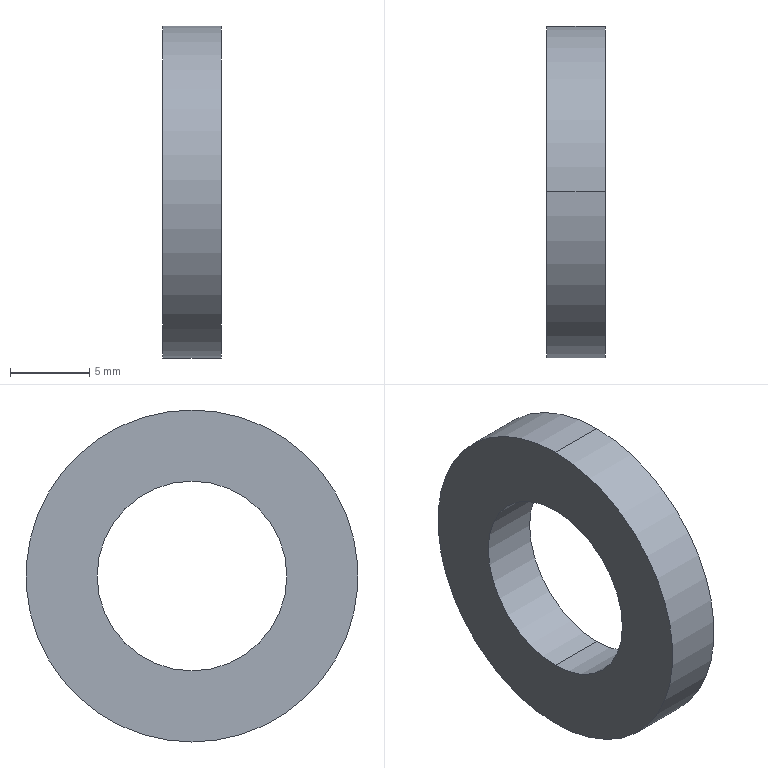Part | STEP file | LHBBW12collar3_Default | 1 solid | 6 faces | box 3.7 x 21 x 21 mm | volume 863.074 mm3 | cylinder 4 | plane 2 | commonest cylinder face diameters 12 x2 21 x2
STEP:
#1=CARTESIAN_POINT('',(0.,0.,0.));
#2=DIRECTION('',(0.,0.,1.));
#3=DIRECTION('',(1.,0.,0.));
#4=AXIS2_PLACEMENT_3D('',#1,#2,#3);
#5=CARTESIAN_POINT('',(1.85,0.,6.));
#6=VERTEX_POINT('',#5);
#7=CARTESIAN_POINT('',(-1.85,0.,6.));
#8=VERTEX_POINT('',#7);
#9=CARTESIAN_POINT('',(1.85,0.,6.));
#10=DIRECTION('',(-1.,0.,0.));
#11=VECTOR('',#10,1.);
#12=LINE('',#9,#11);
#13=CARTESIAN_POINT('',(1.85,0.,0.));
#14=DIRECTION('',(-1.,0.,0.));
#15=DIRECTION('',(0.,0.,1.));
#16=AXIS2_PLACEMENT_3D('',#13,#14,#15);
#17=CYLINDRICAL_SURFACE('',#16,6.);
#18=CARTESIAN_POINT('',(6.283,0.));
#19=DIRECTION('',(0.,1.));
#20=VECTOR('',#19,1.);
#21=LINE('',#18,#20);
#22=(GEOMETRIC_REPRESENTATION_CONTEXT(2)PARAMETRIC_REPRESENTATION_CONTEXT()REPRESENTATION_CONTEXT('',''));
#23=DEFINITIONAL_REPRESENTATION('',(#21),#22);
#24=PCURVE('',#17,#23);
#25=CARTESIAN_POINT('',(1.85,0.,0.));
#26=DIRECTION('',(-1.,0.,0.));
#27=DIRECTION('',(0.,0.,1.));
#28=AXIS2_PLACEMENT_3D('',#25,#26,#27);
#29=CYLINDRICAL_SURFACE('',#28,6.);
#30=CARTESIAN_POINT('',(0.,0.));
#31=DIRECTION('',(0.,1.));
#32=VECTOR('',#31,1.);
#33=LINE('',#30,#32);
#34=(GEOMETRIC_REPRESENTATION_CONTEXT(2)PARAMETRIC_REPRESENTATION_CONTEXT()REPRESENTATION_CONTEXT('',''));
#35=DEFINITIONAL_REPRESENTATION('',(#33),#34);
#36=PCURVE('',#29,#35);
#37=SURFACE_CURVE('',#12,(#24,#36),.PCURVE_S1.);
#38=EDGE_CURVE('',#6,#8,#37,.T.);
#39=ORIENTED_EDGE('',*,*,#38,.T.);
#40=CARTESIAN_POINT('',(-1.85,0.,-6.));
#41=VERTEX_POINT('',#40);
#42=CARTESIAN_POINT('',(-1.85,0.,0.));
#43=DIRECTION('',(-1.,0.,0.));
#44=DIRECTION('',(0.,0.,1.));
#45=AXIS2_PLACEMENT_3D('',#42,#43,#44);
#46=CIRCLE('',#45,6.);
#47=CARTESIAN_POINT('',(0.,3.7));
#48=DIRECTION('',(1.,0.));
#49=VECTOR('',#48,1.);
#50=LINE('',#47,#49);
#51=(GEOMETRIC_REPRESENTATION_CONTEXT(2)PARAMETRIC_REPRESENTATION_CONTEXT()REPRESENTATION_CONTEXT('',''));
#52=DEFINITIONAL_REPRESENTATION('',(#50),#51);
#53=PCURVE('',#17,#52);
#54=CARTESIAN_POINT('',(-1.85,10.5,0.));
#55=DIRECTION('',(1.,0.,0.));
#56=DIRECTION('',(0.,0.,-1.));
#57=AXIS2_PLACEMENT_3D('',#54,#55,#56);
#58=PLANE('',#57);
#59=CARTESIAN_POINT('',(-6.,-10.5));
#60=CARTESIAN_POINT('',(-6.,-0.1077));
#61=CARTESIAN_POINT('',(3.,-5.304));
#62=CARTESIAN_POINT('',(12.,-10.5));
#63=CARTESIAN_POINT('',(3.,-15.696));
#64=CARTESIAN_POINT('',(-6.,-20.892));
#65=CARTESIAN_POINT('',(-6.,-10.5));
#66=(BOUNDED_CURVE()B_SPLINE_CURVE(2,(#59,#60,#61,#62,#63,#64,#65),.UNSPECIFIED.,.T.,.F.)B_SPLINE_CURVE_WITH_KNOTS((1,2,2,2,2,1),(-2.094,0.,2.094,4.189,6.283,8.378),.UNSPECIFIED.)CURVE()GEOMETRIC_REPRESENTATION_ITEM()RATIONAL_B_SPLINE_CURVE((1.,0.5,1.,0.5,1.,0.5,1.))REPRESENTATION_ITEM(''));
#67=(GEOMETRIC_REPRESENTATION_CONTEXT(2)PARAMETRIC_REPRESENTATION_CONTEXT()REPRESENTATION_CONTEXT('',''));
#68=DEFINITIONAL_REPRESENTATION('',(#66),#67);
#69=PCURVE('',#58,#68);
#70=SURFACE_CURVE('',#46,(#53,#69),.PCURVE_S1.);
#71=EDGE_CURVE('',#41,#8,#70,.T.);
#72=ORIENTED_EDGE('',*,*,#71,.F.);
#73=CARTESIAN_POINT('',(1.85,0.,-6.));
#74=VERTEX_POINT('',#73);
#75=CARTESIAN_POINT('',(1.85,0.,-6.));
#76=DIRECTION('',(-1.,0.,0.));
#77=VECTOR('',#76,1.);
#78=LINE('',#75,#77);
#79=CARTESIAN_POINT('',(3.142,0.));
#80=DIRECTION('',(0.,1.));
#81=VECTOR('',#80,1.);
#82=LINE('',#79,#81);
#83=(GEOMETRIC_REPRESENTATION_CONTEXT(2)PARAMETRIC_REPRESENTATION_CONTEXT()REPRESENTATION_CONTEXT('',''));
#84=DEFINITIONAL_REPRESENTATION('',(#82),#83);
#85=PCURVE('',#17,#84);
#86=CARTESIAN_POINT('',(3.142,0.));
#87=DIRECTION('',(0.,1.));
#88=VECTOR('',#87,1.);
#89=LINE('',#86,#88);
#90=(GEOMETRIC_REPRESENTATION_CONTEXT(2)PARAMETRIC_REPRESENTATION_CONTEXT()REPRESENTATION_CONTEXT('',''));
#91=DEFINITIONAL_REPRESENTATION('',(#89),#90);
#92=PCURVE('',#29,#91);
#93=SURFACE_CURVE('',#78,(#85,#92),.PCURVE_S1.);
#94=EDGE_CURVE('',#74,#41,#93,.T.);
#95=ORIENTED_EDGE('',*,*,#94,.F.);
#96=CARTESIAN_POINT('',(1.85,0.,0.));
#97=DIRECTION('',(-1.,0.,0.));
#98=DIRECTION('',(0.,0.,1.));
#99=AXIS2_PLACEMENT_3D('',#96,#97,#98);
#100=CIRCLE('',#99,6.);
#101=CARTESIAN_POINT('',(0.,0.));
#102=DIRECTION('',(1.,0.));
#103=VECTOR('',#102,1.);
#104=LINE('',#101,#103);
#105=(GEOMETRIC_REPRESENTATION_CONTEXT(2)PARAMETRIC_REPRESENTATION_CONTEXT()REPRESENTATION_CONTEXT('',''));
#106=DEFINITIONAL_REPRESENTATION('',(#104),#105);
#107=PCURVE('',#17,#106);
#108=CARTESIAN_POINT('',(1.85,6.,0.));
#109=DIRECTION('',(-1.,0.,0.));
#110=DIRECTION('',(0.,0.,1.));
#111=AXIS2_PLACEMENT_3D('',#108,#109,#110);
#112=PLANE('',#111);
#113=CARTESIAN_POINT('',(0.,-6.));
#114=DIRECTION('',(1.,0.));
#115=AXIS2_PLACEMENT_2D('',#113,#114);
#116=CIRCLE('',#115,6.);
#117=(GEOMETRIC_REPRESENTATION_CONTEXT(2)PARAMETRIC_REPRESENTATION_CONTEXT()REPRESENTATION_CONTEXT('',''));
#118=DEFINITIONAL_REPRESENTATION('',(#116),#117);
#119=PCURVE('',#112,#118);
#120=SURFACE_CURVE('',#100,(#107,#119),.PCURVE_S1.);
#121=EDGE_CURVE('',#74,#6,#120,.T.);
#122=ORIENTED_EDGE('',*,*,#121,.T.);
#123=EDGE_LOOP('',(#39,#72,#95,#122));
#124=FACE_BOUND('',#123,.F.);
#125=ADVANCED_FACE('',(#124),#17,.F.);
#126=CARTESIAN_POINT('',(1.85,0.,10.5));
#127=VERTEX_POINT('',#126);
#128=CARTESIAN_POINT('',(1.85,0.,-10.5));
#129=VERTEX_POINT('',#128);
#130=CARTESIAN_POINT('',(1.85,0.,0.));
#131=DIRECTION('',(-1.,0.,0.));
#132=DIRECTION('',(0.,0.,1.));
#133=AXIS2_PLACEMENT_3D('',#130,#131,#132);
#134=CIRCLE('',#133,10.5);
#135=CARTESIAN_POINT('',(1.85,0.,0.));
#136=DIRECTION('',(-1.,0.,0.));
#137=DIRECTION('',(0.,0.,1.));
#138=AXIS2_PLACEMENT_3D('',#135,#136,#137);
#139=CYLINDRICAL_SURFACE('',#138,10.5);
#140=CARTESIAN_POINT('',(0.,0.));
#141=DIRECTION('',(1.,0.));
#142=VECTOR('',#141,1.);
#143=LINE('',#140,#142);
#144=(GEOMETRIC_REPRESENTATION_CONTEXT(2)PARAMETRIC_REPRESENTATION_CONTEXT()REPRESENTATION_CONTEXT('',''));
#145=DEFINITIONAL_REPRESENTATION('',(#143),#144);
#146=PCURVE('',#139,#145);
#147=CARTESIAN_POINT('',(0.,-6.));
#148=DIRECTION('',(1.,0.));
#149=AXIS2_PLACEMENT_2D('',#147,#148);
#150=CIRCLE('',#149,10.5);
#151=(GEOMETRIC_REPRESENTATION_CONTEXT(2)PARAMETRIC_REPRESENTATION_CONTEXT()REPRESENTATION_CONTEXT('',''));
#152=DEFINITIONAL_REPRESENTATION('',(#150),#151);
#153=PCURVE('',#112,#152);
#154=SURFACE_CURVE('',#134,(#146,#153),.PCURVE_S1.);
#155=EDGE_CURVE('',#127,#129,#154,.T.);
#156=ORIENTED_EDGE('',*,*,#155,.T.);
#157=CARTESIAN_POINT('',(-1.85,0.,-10.5));
#158=VERTEX_POINT('',#157);
#159=CARTESIAN_POINT('',(1.85,0.,-10.5));
#160=DIRECTION('',(-1.,0.,0.));
#161=VECTOR('',#160,1.);
#162=LINE('',#159,#161);
#163=CARTESIAN_POINT('',(3.142,0.));
#164=DIRECTION('',(0.,1.));
#165=VECTOR('',#164,1.);
#166=LINE('',#163,#165);
#167=(GEOMETRIC_REPRESENTATION_CONTEXT(2)PARAMETRIC_REPRESENTATION_CONTEXT()REPRESENTATION_CONTEXT('',''));
#168=DEFINITIONAL_REPRESENTATION('',(#166),#167);
#169=PCURVE('',#139,#168);
#170=CARTESIAN_POINT('',(1.85,0.,0.));
#171=DIRECTION('',(-1.,0.,0.));
#172=DIRECTION('',(0.,0.,1.));
#173=AXIS2_PLACEMENT_3D('',#170,#171,#172);
#174=CYLINDRICAL_SURFACE('',#173,10.5);
#175=CARTESIAN_POINT('',(3.142,0.));
#176=DIRECTION('',(0.,1.));
#177=VECTOR('',#176,1.);
#178=LINE('',#175,#177);
#179=(GEOMETRIC_REPRESENTATION_CONTEXT(2)PARAMETRIC_REPRESENTATION_CONTEXT()REPRESENTATION_CONTEXT('',''));
#180=DEFINITIONAL_REPRESENTATION('',(#178),#179);
#181=PCURVE('',#174,#180);
#182=SURFACE_CURVE('',#162,(#169,#181),.PCURVE_S1.);
#183=EDGE_CURVE('',#129,#158,#182,.T.);
#184=ORIENTED_EDGE('',*,*,#183,.T.);
#185=CARTESIAN_POINT('',(-1.85,0.,10.5));
#186=VERTEX_POINT('',#185);
#187=CARTESIAN_POINT('',(-1.85,0.,0.));
#188=DIRECTION('',(-1.,0.,0.));
#189=DIRECTION('',(0.,0.,1.));
#190=AXIS2_PLACEMENT_3D('',#187,#188,#189);
#191=CIRCLE('',#190,10.5);
#192=CARTESIAN_POINT('',(0.,3.7));
#193=DIRECTION('',(1.,0.));
#194=VECTOR('',#193,1.);
#195=LINE('',#192,#194);
#196=(GEOMETRIC_REPRESENTATION_CONTEXT(2)PARAMETRIC_REPRESENTATION_CONTEXT()REPRESENTATION_CONTEXT('',''));
#197=DEFINITIONAL_REPRESENTATION('',(#195),#196);
#198=PCURVE('',#139,#197);
#199=CARTESIAN_POINT('',(-10.5,-10.5));
#200=CARTESIAN_POINT('',(-10.5,7.687));
#201=CARTESIAN_POINT('',(5.25,-1.407));
#202=CARTESIAN_POINT('',(21.,-10.5));
#203=CARTESIAN_POINT('',(5.25,-19.593));
#204=CARTESIAN_POINT('',(-10.5,-28.687));
#205=CARTESIAN_POINT('',(-10.5,-10.5));
#206=(BOUNDED_CURVE()B_SPLINE_CURVE(2,(#199,#200,#201,#202,#203,#204,#205),.UNSPECIFIED.,.T.,.F.)B_SPLINE_CURVE_WITH_KNOTS((1,2,2,2,2,1),(-2.094,0.,2.094,4.189,6.283,8.378),.UNSPECIFIED.)CURVE()GEOMETRIC_REPRESENTATION_ITEM()RATIONAL_B_SPLINE_CURVE((1.,0.5,1.,0.5,1.,0.5,1.))REPRESENTATION_ITEM(''));
#207=(GEOMETRIC_REPRESENTATION_CONTEXT(2)PARAMETRIC_REPRESENTATION_CONTEXT()REPRESENTATION_CONTEXT('',''));
#208=DEFINITIONAL_REPRESENTATION('',(#206),#207);
#209=PCURVE('',#58,#208);
#210=SURFACE_CURVE('',#191,(#198,#209),.PCURVE_S1.);
#211=EDGE_CURVE('',#186,#158,#210,.T.);
#212=ORIENTED_EDGE('',*,*,#211,.F.);
#213=CARTESIAN_POINT('',(1.85,0.,10.5));
#214=DIRECTION('',(-1.,0.,0.));
#215=VECTOR('',#214,1.);
#216=LINE('',#213,#215);
#217=CARTESIAN_POINT('',(0.,0.));
#218=DIRECTION('',(0.,1.));
#219=VECTOR('',#218,1.);
#220=LINE('',#217,#219);
#221=(GEOMETRIC_REPRESENTATION_CONTEXT(2)PARAMETRIC_REPRESENTATION_CONTEXT()REPRESENTATION_CONTEXT('',''));
#222=DEFINITIONAL_REPRESENTATION('',(#220),#221);
#223=PCURVE('',#139,#222);
#224=CARTESIAN_POINT('',(6.283,0.));
#225=DIRECTION('',(0.,1.));
#226=VECTOR('',#225,1.);
#227=LINE('',#224,#226);
#228=(GEOMETRIC_REPRESENTATION_CONTEXT(2)PARAMETRIC_REPRESENTATION_CONTEXT()REPRESENTATION_CONTEXT('',''));
#229=DEFINITIONAL_REPRESENTATION('',(#227),#228);
#230=PCURVE('',#174,#229);
#231=SURFACE_CURVE('',#216,(#223,#230),.PCURVE_S1.);
#232=EDGE_CURVE('',#127,#186,#231,.T.);
#233=ORIENTED_EDGE('',*,*,#232,.F.);
#234=EDGE_LOOP('',(#156,#184,#212,#233));
#235=FACE_BOUND('',#234,.T.);
#236=ADVANCED_FACE('',(#235),#139,.T.);
#237=ORIENTED_EDGE('',*,*,#183,.F.);
#238=CARTESIAN_POINT('',(1.85,0.,0.));
#239=DIRECTION('',(-1.,0.,0.));
#240=DIRECTION('',(0.,0.,1.));
#241=AXIS2_PLACEMENT_3D('',#238,#239,#240);
#242=CIRCLE('',#241,10.5);
#243=CARTESIAN_POINT('',(0.,0.));
#244=DIRECTION('',(1.,0.));
#245=VECTOR('',#244,1.);
#246=LINE('',#243,#245);
#247=(GEOMETRIC_REPRESENTATION_CONTEXT(2)PARAMETRIC_REPRESENTATION_CONTEXT()REPRESENTATION_CONTEXT('',''));
#248=DEFINITIONAL_REPRESENTATION('',(#246),#247);
#249=PCURVE('',#174,#248);
#250=CARTESIAN_POINT('',(0.,-6.));
#251=DIRECTION('',(1.,0.));
#252=AXIS2_PLACEMENT_2D('',#250,#251);
#253=CIRCLE('',#252,10.5);
#254=(GEOMETRIC_REPRESENTATION_CONTEXT(2)PARAMETRIC_REPRESENTATION_CONTEXT()REPRESENTATION_CONTEXT('',''));
#255=DEFINITIONAL_REPRESENTATION('',(#253),#254);
#256=PCURVE('',#112,#255);
#257=SURFACE_CURVE('',#242,(#249,#256),.PCURVE_S1.);
#258=EDGE_CURVE('',#129,#127,#257,.T.);
#259=ORIENTED_EDGE('',*,*,#258,.T.);
#260=ORIENTED_EDGE('',*,*,#232,.T.);
#261=CARTESIAN_POINT('',(-1.85,0.,0.));
#262=DIRECTION('',(-1.,0.,0.));
#263=DIRECTION('',(0.,0.,1.));
#264=AXIS2_PLACEMENT_3D('',#261,#262,#263);
#265=CIRCLE('',#264,10.5);
#266=CARTESIAN_POINT('',(0.,3.7));
#267=DIRECTION('',(1.,0.));
#268=VECTOR('',#267,1.);
#269=LINE('',#266,#268);
#270=(GEOMETRIC_REPRESENTATION_CONTEXT(2)PARAMETRIC_REPRESENTATION_CONTEXT()REPRESENTATION_CONTEXT('',''));
#271=DEFINITIONAL_REPRESENTATION('',(#269),#270);
#272=PCURVE('',#174,#271);
#273=CARTESIAN_POINT('',(-10.5,-10.5));
#274=CARTESIAN_POINT('',(-10.5,7.687));
#275=CARTESIAN_POINT('',(5.25,-1.407));
#276=CARTESIAN_POINT('',(21.,-10.5));
#277=CARTESIAN_POINT('',(5.25,-19.593));
#278=CARTESIAN_POINT('',(-10.5,-28.687));
#279=CARTESIAN_POINT('',(-10.5,-10.5));
#280=(BOUNDED_CURVE()B_SPLINE_CURVE(2,(#273,#274,#275,#276,#277,#278,#279),.UNSPECIFIED.,.T.,.F.)B_SPLINE_CURVE_WITH_KNOTS((1,2,2,2,2,1),(-2.094,0.,2.094,4.189,6.283,8.378),.UNSPECIFIED.)CURVE()GEOMETRIC_REPRESENTATION_ITEM()RATIONAL_B_SPLINE_CURVE((1.,0.5,1.,0.5,1.,0.5,1.))REPRESENTATION_ITEM(''));
#281=(GEOMETRIC_REPRESENTATION_CONTEXT(2)PARAMETRIC_REPRESENTATION_CONTEXT()REPRESENTATION_CONTEXT('',''));
#282=DEFINITIONAL_REPRESENTATION('',(#280),#281);
#283=PCURVE('',#58,#282);
#284=SURFACE_CURVE('',#265,(#272,#283),.PCURVE_S1.);
#285=EDGE_CURVE('',#158,#186,#284,.T.);
#286=ORIENTED_EDGE('',*,*,#285,.F.);
#287=EDGE_LOOP('',(#237,#259,#260,#286));
#288=FACE_BOUND('',#287,.T.);
#289=ADVANCED_FACE('',(#288),#174,.T.);
#290=CARTESIAN_POINT('',(-1.85,0.,0.));
#291=DIRECTION('',(-1.,0.,0.));
#292=DIRECTION('',(0.,0.,1.));
#293=AXIS2_PLACEMENT_3D('',#290,#291,#292);
#294=CIRCLE('',#293,6.);
#295=CARTESIAN_POINT('',(-6.,-10.5));
#296=CARTESIAN_POINT('',(-6.,-0.1077));
#297=CARTESIAN_POINT('',(3.,-5.304));
#298=CARTESIAN_POINT('',(12.,-10.5));
#299=CARTESIAN_POINT('',(3.,-15.696));
#300=CARTESIAN_POINT('',(-6.,-20.892));
#301=CARTESIAN_POINT('',(-6.,-10.5));
#302=(BOUNDED_CURVE()B_SPLINE_CURVE(2,(#295,#296,#297,#298,#299,#300,#301),.UNSPECIFIED.,.T.,.F.)B_SPLINE_CURVE_WITH_KNOTS((1,2,2,2,2,1),(-2.094,0.,2.094,4.189,6.283,8.378),.UNSPECIFIED.)CURVE()GEOMETRIC_REPRESENTATION_ITEM()RATIONAL_B_SPLINE_CURVE((1.,0.5,1.,0.5,1.,0.5,1.))REPRESENTATION_ITEM(''));
#303=(GEOMETRIC_REPRESENTATION_CONTEXT(2)PARAMETRIC_REPRESENTATION_CONTEXT()REPRESENTATION_CONTEXT('',''));
#304=DEFINITIONAL_REPRESENTATION('',(#302),#303);
#305=PCURVE('',#58,#304);
#306=CARTESIAN_POINT('',(0.,3.7));
#307=DIRECTION('',(1.,0.));
#308=VECTOR('',#307,1.);
#309=LINE('',#306,#308);
#310=(GEOMETRIC_REPRESENTATION_CONTEXT(2)PARAMETRIC_REPRESENTATION_CONTEXT()REPRESENTATION_CONTEXT('',''));
#311=DEFINITIONAL_REPRESENTATION('',(#309),#310);
#312=PCURVE('',#29,#311);
#313=SURFACE_CURVE('',#294,(#305,#312),.PCURVE_S1.);
#314=EDGE_CURVE('',#8,#41,#313,.T.);
#315=ORIENTED_EDGE('',*,*,#314,.F.);
#316=ORIENTED_EDGE('',*,*,#71,.F.);
#317=EDGE_LOOP('',(#315,#316));
#318=FACE_BOUND('',#317,.T.);
#319=ORIENTED_EDGE('',*,*,#211,.T.);
#320=ORIENTED_EDGE('',*,*,#285,.T.);
#321=EDGE_LOOP('',(#319,#320));
#322=FACE_BOUND('',#321,.T.);
#323=ADVANCED_FACE('',(#318,#322),#58,.F.);
#324=ORIENTED_EDGE('',*,*,#314,.F.);
#325=ORIENTED_EDGE('',*,*,#38,.F.);
#326=CARTESIAN_POINT('',(1.85,0.,0.));
#327=DIRECTION('',(-1.,0.,0.));
#328=DIRECTION('',(0.,0.,1.));
#329=AXIS2_PLACEMENT_3D('',#326,#327,#328);
#330=CIRCLE('',#329,6.);
#331=CARTESIAN_POINT('',(0.,0.));
#332=DIRECTION('',(1.,0.));
#333=VECTOR('',#332,1.);
#334=LINE('',#331,#333);
#335=(GEOMETRIC_REPRESENTATION_CONTEXT(2)PARAMETRIC_REPRESENTATION_CONTEXT()REPRESENTATION_CONTEXT('',''));
#336=DEFINITIONAL_REPRESENTATION('',(#334),#335);
#337=PCURVE('',#29,#336);
#338=CARTESIAN_POINT('',(0.,-6.));
#339=DIRECTION('',(1.,0.));
#340=AXIS2_PLACEMENT_2D('',#338,#339);
#341=CIRCLE('',#340,6.);
#342=(GEOMETRIC_REPRESENTATION_CONTEXT(2)PARAMETRIC_REPRESENTATION_CONTEXT()REPRESENTATION_CONTEXT('',''));
#343=DEFINITIONAL_REPRESENTATION('',(#341),#342);
#344=PCURVE('',#112,#343);
#345=SURFACE_CURVE('',#330,(#337,#344),.PCURVE_S1.);
#346=EDGE_CURVE('',#6,#74,#345,.T.);
#347=ORIENTED_EDGE('',*,*,#346,.T.);
#348=ORIENTED_EDGE('',*,*,#94,.T.);
#349=EDGE_LOOP('',(#324,#325,#347,#348));
#350=FACE_BOUND('',#349,.F.);
#351=ADVANCED_FACE('',(#350),#29,.F.);
#352=ORIENTED_EDGE('',*,*,#155,.F.);
#353=ORIENTED_EDGE('',*,*,#258,.F.);
#354=EDGE_LOOP('',(#352,#353));
#355=FACE_BOUND('',#354,.T.);
#356=ORIENTED_EDGE('',*,*,#346,.T.);
#357=ORIENTED_EDGE('',*,*,#121,.T.);
#358=EDGE_LOOP('',(#356,#357));
#359=FACE_BOUND('',#358,.T.);
#360=ADVANCED_FACE('',(#355,#359),#112,.F.);
#361=CLOSED_SHELL('',(#125,#236,#289,#323,#351,#360));
#362=MANIFOLD_SOLID_BREP('',#361);
#363=(LENGTH_UNIT()NAMED_UNIT(*)SI_UNIT(.MILLI.,.METRE.));
#364=UNCERTAINTY_MEASURE_WITH_UNIT(LENGTH_MEASURE(0.0000001),#363,'','');
#365=(NAMED_UNIT(*)PLANE_ANGLE_UNIT()SI_UNIT($,.RADIAN.));
#366=(NAMED_UNIT(*)SI_UNIT($,.STERADIAN.)SOLID_ANGLE_UNIT());
#367=(GEOMETRIC_REPRESENTATION_CONTEXT(3)GLOBAL_UNCERTAINTY_ASSIGNED_CONTEXT((#364))GLOBAL_UNIT_ASSIGNED_CONTEXT((#363,#365,#366))REPRESENTATION_CONTEXT('',''));
#368=ADVANCED_BREP_SHAPE_REPRESENTATION('',(#4,#362),#367);